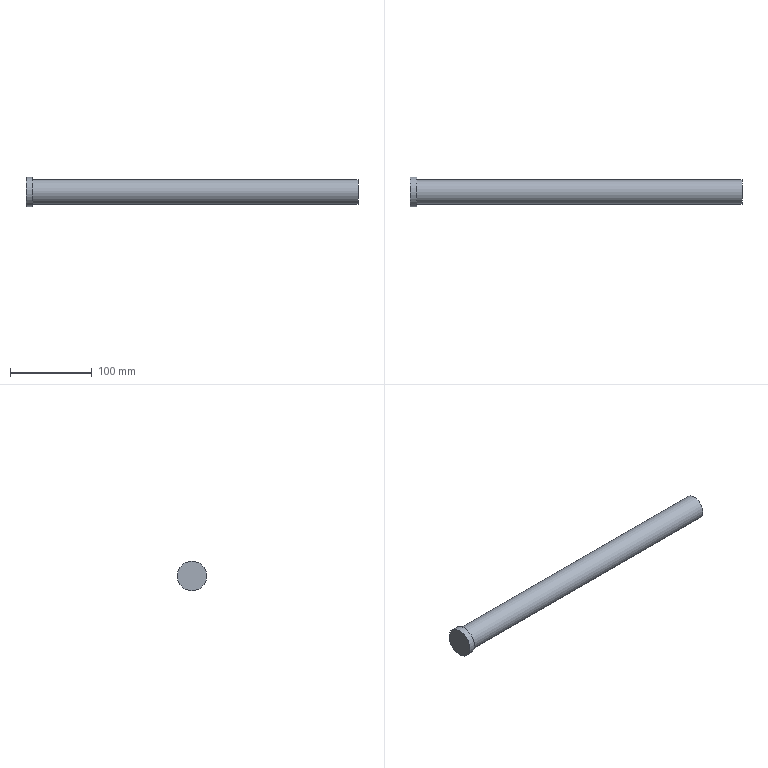Part | STEP file | solid 55 | 1 solid | 8 faces | box 406 x 36 x 36 mm | volume 287307 mm3 | plane 4 | cylinder 3 | cone 1 | commonest cylinder face diameters 10.5 x1 30 x1 36 x1